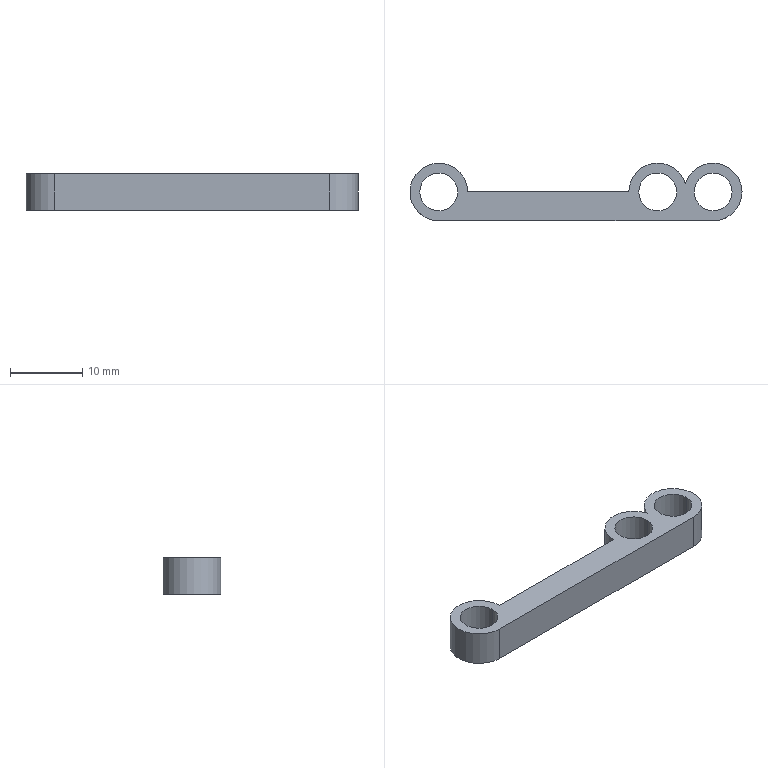Part | SolidWorks | features ICE 13, RevCut 2, Attribute 1, Extrusion 1 | 1 solid | 14 faces | box 46 x 8 x 5 mm | volume 936.72 mm3 | cylinder 10 | plane 4 | commonest cylinder face diameters 5.25 x6 8 x4
STEP:
#1=CARTESIAN_POINT('',(2.051,-2.5,0.));
#2=VERTEX_POINT('',#1);
#3=CARTESIAN_POINT('',(7.301,-2.5,0.));
#4=VERTEX_POINT('',#3);
#5=CARTESIAN_POINT('',(4.676,-2.5,0.));
#6=DIRECTION('',(0.,0.,1.));
#7=DIRECTION('',(1.,0.,0.));
#8=AXIS2_PLACEMENT_3D('',#5,#6,#7);
#9=CIRCLE('',#8,2.625);
#10=EDGE_CURVE('',#2,#4,#9,.T.);
#11=ORIENTED_EDGE('',*,*,#10,.F.);
#12=CARTESIAN_POINT('',(2.051,-2.5,5.));
#13=VERTEX_POINT('',#12);
#14=CARTESIAN_POINT('',(2.051,-2.5,-5.));
#15=DIRECTION('',(0.,0.,1.));
#16=VECTOR('',#15,1000.);
#17=LINE('',#14,#16);
#18=EDGE_CURVE('',#2,#13,#17,.T.);
#19=ORIENTED_EDGE('',*,*,#18,.T.);
#20=CARTESIAN_POINT('',(7.301,-2.5,5.));
#21=VERTEX_POINT('',#20);
#22=CARTESIAN_POINT('',(4.676,-2.5,5.));
#23=DIRECTION('',(0.,0.,1.));
#24=DIRECTION('',(1.,0.,0.));
#25=AXIS2_PLACEMENT_3D('',#22,#23,#24);
#26=CIRCLE('',#25,2.625);
#27=EDGE_CURVE('',#13,#21,#26,.T.);
#28=ORIENTED_EDGE('',*,*,#27,.T.);
#29=CARTESIAN_POINT('',(7.301,-2.5,-5.));
#30=DIRECTION('',(0.,0.,1.));
#31=VECTOR('',#30,1000.);
#32=LINE('',#29,#31);
#33=EDGE_CURVE('',#4,#21,#32,.T.);
#34=ORIENTED_EDGE('',*,*,#33,.F.);
#35=EDGE_LOOP('',(#11,#19,#28,#34));
#36=FACE_OUTER_BOUND('',#35,.T.);
#37=CARTESIAN_POINT('',(4.676,-2.5,-5.));
#38=DIRECTION('',(0.,0.,1.));
#39=DIRECTION('',(1.,0.,0.));
#40=AXIS2_PLACEMENT_3D('',#37,#38,#39);
#41=CYLINDRICAL_SURFACE('',#40,2.625);
#42=ADVANCED_FACE('',(#36),#41,.F.);
#43=CARTESIAN_POINT('',(32.375,-2.5,5.));
#44=VERTEX_POINT('',#43);
#45=CARTESIAN_POINT('',(37.625,-2.5,5.));
#46=VERTEX_POINT('',#45);
#47=CARTESIAN_POINT('',(35.,-2.5,5.));
#48=DIRECTION('',(0.,0.,1.));
#49=DIRECTION('',(1.,0.,0.));
#50=AXIS2_PLACEMENT_3D('',#47,#48,#49);
#51=CIRCLE('',#50,2.625);
#52=EDGE_CURVE('',#44,#46,#51,.T.);
#53=ORIENTED_EDGE('',*,*,#52,.T.);
#54=CARTESIAN_POINT('',(37.625,-2.5,0.));
#55=VERTEX_POINT('',#54);
#56=CARTESIAN_POINT('',(37.625,-2.5,14.));
#57=DIRECTION('',(0.,0.,-1.));
#58=VECTOR('',#57,1000.);
#59=LINE('',#56,#58);
#60=EDGE_CURVE('',#46,#55,#59,.T.);
#61=ORIENTED_EDGE('',*,*,#60,.T.);
#62=CARTESIAN_POINT('',(32.375,-2.5,0.));
#63=VERTEX_POINT('',#62);
#64=CARTESIAN_POINT('',(35.,-2.5,0.));
#65=DIRECTION('',(0.,0.,-1.));
#66=DIRECTION('',(-1.,0.,0.));
#67=AXIS2_PLACEMENT_3D('',#64,#65,#66);
#68=CIRCLE('',#67,2.625);
#69=EDGE_CURVE('',#55,#63,#68,.T.);
#70=ORIENTED_EDGE('',*,*,#69,.T.);
#71=CARTESIAN_POINT('',(32.375,-2.5,14.));
#72=DIRECTION('',(0.,0.,-1.));
#73=VECTOR('',#72,1000.);
#74=LINE('',#71,#73);
#75=EDGE_CURVE('',#44,#63,#74,.T.);
#76=ORIENTED_EDGE('',*,*,#75,.F.);
#77=EDGE_LOOP('',(#53,#61,#70,#76));
#78=FACE_OUTER_BOUND('',#77,.T.);
#79=CARTESIAN_POINT('',(35.,-2.5,14.));
#80=DIRECTION('',(0.,0.,-1.));
#81=DIRECTION('',(-1.,0.,0.));
#82=AXIS2_PLACEMENT_3D('',#79,#80,#81);
#83=CYLINDRICAL_SURFACE('',#82,2.625);
#84=ADVANCED_FACE('',(#78),#83,.F.);
#85=CARTESIAN_POINT('',(40.051,-2.5,0.));
#86=VERTEX_POINT('',#85);
#87=CARTESIAN_POINT('',(45.301,-2.5,0.));
#88=VERTEX_POINT('',#87);
#89=CARTESIAN_POINT('',(42.676,-2.5,0.));
#90=DIRECTION('',(0.,0.,1.));
#91=DIRECTION('',(1.,0.,0.));
#92=AXIS2_PLACEMENT_3D('',#89,#90,#91);
#93=CIRCLE('',#92,2.625);
#94=EDGE_CURVE('',#86,#88,#93,.T.);
#95=ORIENTED_EDGE('',*,*,#94,.F.);
#96=CARTESIAN_POINT('',(40.051,-2.5,5.));
#97=VERTEX_POINT('',#96);
#98=CARTESIAN_POINT('',(40.051,-2.5,-2.));
#99=DIRECTION('',(0.,0.,1.));
#100=VECTOR('',#99,1000.);
#101=LINE('',#98,#100);
#102=EDGE_CURVE('',#86,#97,#101,.T.);
#103=ORIENTED_EDGE('',*,*,#102,.T.);
#104=CARTESIAN_POINT('',(45.301,-2.5,5.));
#105=VERTEX_POINT('',#104);
#106=CARTESIAN_POINT('',(42.676,-2.5,5.));
#107=DIRECTION('',(0.,0.,1.));
#108=DIRECTION('',(1.,0.,0.));
#109=AXIS2_PLACEMENT_3D('',#106,#107,#108);
#110=CIRCLE('',#109,2.625);
#111=EDGE_CURVE('',#97,#105,#110,.T.);
#112=ORIENTED_EDGE('',*,*,#111,.T.);
#113=CARTESIAN_POINT('',(45.301,-2.5,-2.));
#114=DIRECTION('',(0.,0.,1.));
#115=VECTOR('',#114,1000.);
#116=LINE('',#113,#115);
#117=EDGE_CURVE('',#88,#105,#116,.T.);
#118=ORIENTED_EDGE('',*,*,#117,.F.);
#119=EDGE_LOOP('',(#95,#103,#112,#118));
#120=FACE_OUTER_BOUND('',#119,.T.);
#121=CARTESIAN_POINT('',(42.676,-2.5,-2.));
#122=DIRECTION('',(0.,0.,1.));
#123=DIRECTION('',(1.,0.,0.));
#124=AXIS2_PLACEMENT_3D('',#121,#122,#123);
#125=CYLINDRICAL_SURFACE('',#124,2.625);
#126=ADVANCED_FACE('',(#120),#125,.F.);
#127=CARTESIAN_POINT('',(42.676,-6.5,0.));
#128=VERTEX_POINT('',#127);
#129=CARTESIAN_POINT('',(46.676,-2.5,0.));
#130=VERTEX_POINT('',#129);
#131=CARTESIAN_POINT('',(42.676,-2.5,0.));
#132=DIRECTION('',(0.,0.,1.));
#133=DIRECTION('',(1.,0.,0.));
#134=AXIS2_PLACEMENT_3D('',#131,#132,#133);
#135=CIRCLE('',#134,4.);
#136=EDGE_CURVE('',#128,#130,#135,.T.);
#137=ORIENTED_EDGE('',*,*,#136,.T.);
#138=CARTESIAN_POINT('',(46.676,-2.5,5.));
#139=VERTEX_POINT('',#138);
#140=CARTESIAN_POINT('',(46.676,-2.5,0.));
#141=DIRECTION('',(0.,0.,1.));
#142=VECTOR('',#141,1000.);
#143=LINE('',#140,#142);
#144=EDGE_CURVE('',#130,#139,#143,.T.);
#145=ORIENTED_EDGE('',*,*,#144,.T.);
#146=CARTESIAN_POINT('',(42.676,-6.5,5.));
#147=VERTEX_POINT('',#146);
#148=CARTESIAN_POINT('',(42.676,-2.5,5.));
#149=DIRECTION('',(0.,0.,1.));
#150=DIRECTION('',(1.,0.,0.));
#151=AXIS2_PLACEMENT_3D('',#148,#149,#150);
#152=CIRCLE('',#151,4.);
#153=EDGE_CURVE('',#147,#139,#152,.T.);
#154=ORIENTED_EDGE('',*,*,#153,.F.);
#155=CARTESIAN_POINT('',(42.676,-6.5,0.));
#156=DIRECTION('',(0.,0.,1.));
#157=VECTOR('',#156,1000.);
#158=LINE('',#155,#157);
#159=EDGE_CURVE('',#128,#147,#158,.T.);
#160=ORIENTED_EDGE('',*,*,#159,.F.);
#161=EDGE_LOOP('',(#137,#145,#154,#160));
#162=FACE_OUTER_BOUND('',#161,.T.);
#163=CARTESIAN_POINT('',(42.676,-2.5,0.));
#164=DIRECTION('',(0.,0.,1.));
#165=DIRECTION('',(1.,0.,0.));
#166=AXIS2_PLACEMENT_3D('',#163,#164,#165);
#167=CYLINDRICAL_SURFACE('',#166,4.);
#168=ADVANCED_FACE('',(#162),#167,.T.);
#169=ORIENTED_EDGE('',*,*,#144,.F.);
#170=CARTESIAN_POINT('',(38.838,-1.373,0.));
#171=VERTEX_POINT('',#170);
#172=CARTESIAN_POINT('',(42.676,-2.5,0.));
#173=DIRECTION('',(0.,0.,1.));
#174=DIRECTION('',(1.,0.,0.));
#175=AXIS2_PLACEMENT_3D('',#172,#173,#174);
#176=CIRCLE('',#175,4.);
#177=EDGE_CURVE('',#130,#171,#176,.T.);
#178=ORIENTED_EDGE('',*,*,#177,.T.);
#179=CARTESIAN_POINT('',(38.838,-1.373,5.));
#180=VERTEX_POINT('',#179);
#181=CARTESIAN_POINT('',(38.838,-1.373,0.));
#182=DIRECTION('',(0.,0.,1.));
#183=VECTOR('',#182,1000.);
#184=LINE('',#181,#183);
#185=EDGE_CURVE('',#171,#180,#184,.T.);
#186=ORIENTED_EDGE('',*,*,#185,.T.);
#187=CARTESIAN_POINT('',(42.676,-2.5,5.));
#188=DIRECTION('',(0.,0.,1.));
#189=DIRECTION('',(1.,0.,0.));
#190=AXIS2_PLACEMENT_3D('',#187,#188,#189);
#191=CIRCLE('',#190,4.);
#192=EDGE_CURVE('',#139,#180,#191,.T.);
#193=ORIENTED_EDGE('',*,*,#192,.F.);
#194=EDGE_LOOP('',(#169,#178,#186,#193));
#195=FACE_OUTER_BOUND('',#194,.T.);
#196=CARTESIAN_POINT('',(42.676,-2.5,0.));
#197=DIRECTION('',(0.,0.,1.));
#198=DIRECTION('',(1.,0.,0.));
#199=AXIS2_PLACEMENT_3D('',#196,#197,#198);
#200=CYLINDRICAL_SURFACE('',#199,4.);
#201=ADVANCED_FACE('',(#195),#200,.T.);
#202=CARTESIAN_POINT('',(8.676,-2.5,5.));
#203=VERTEX_POINT('',#202);
#204=CARTESIAN_POINT('',(4.676,-6.5,5.));
#205=VERTEX_POINT('',#204);
#206=CARTESIAN_POINT('',(4.676,-2.5,5.));
#207=DIRECTION('',(0.,0.,1.));
#208=DIRECTION('',(1.,0.,0.));
#209=AXIS2_PLACEMENT_3D('',#206,#207,#208);
#210=CIRCLE('',#209,4.);
#211=EDGE_CURVE('',#203,#205,#210,.T.);
#212=ORIENTED_EDGE('',*,*,#211,.T.);
#213=CARTESIAN_POINT('',(35.,-6.5,5.));
#214=DIRECTION('',(1.,0.,0.));
#215=VECTOR('',#214,1000.);
#216=LINE('',#213,#215);
#217=EDGE_CURVE('',#205,#147,#216,.T.);
#218=ORIENTED_EDGE('',*,*,#217,.T.);
#219=ORIENTED_EDGE('',*,*,#153,.T.);
#220=ORIENTED_EDGE('',*,*,#192,.T.);
#221=CARTESIAN_POINT('',(31.,-2.5,5.));
#222=VERTEX_POINT('',#221);
#223=CARTESIAN_POINT('',(35.,-2.5,5.));
#224=DIRECTION('',(0.,0.,-1.));
#225=DIRECTION('',(-1.,0.,0.));
#226=AXIS2_PLACEMENT_3D('',#223,#224,#225);
#227=CIRCLE('',#226,4.);
#228=EDGE_CURVE('',#222,#180,#227,.T.);
#229=ORIENTED_EDGE('',*,*,#228,.F.);
#230=CARTESIAN_POINT('',(0.,-2.5,5.));
#231=DIRECTION('',(1.,0.,0.));
#232=VECTOR('',#231,1000.);
#233=LINE('',#230,#232);
#234=EDGE_CURVE('',#203,#222,#233,.T.);
#235=ORIENTED_EDGE('',*,*,#234,.F.);
#236=EDGE_LOOP('',(#212,#218,#219,#220,#229,#235));
#237=FACE_OUTER_BOUND('',#236,.T.);
#238=CARTESIAN_POINT('',(4.676,-2.5,5.));
#239=DIRECTION('',(0.,0.,1.));
#240=DIRECTION('',(1.,0.,0.));
#241=AXIS2_PLACEMENT_3D('',#238,#239,#240);
#242=CIRCLE('',#241,2.625);
#243=EDGE_CURVE('',#21,#13,#242,.T.);
#244=ORIENTED_EDGE('',*,*,#243,.F.);
#245=ORIENTED_EDGE('',*,*,#27,.F.);
#246=EDGE_LOOP('',(#244,#245));
#247=FACE_BOUND('',#246,.T.);
#248=ORIENTED_EDGE('',*,*,#52,.F.);
#249=CARTESIAN_POINT('',(35.,-2.5,5.));
#250=DIRECTION('',(0.,0.,1.));
#251=DIRECTION('',(1.,0.,0.));
#252=AXIS2_PLACEMENT_3D('',#249,#250,#251);
#253=CIRCLE('',#252,2.625);
#254=EDGE_CURVE('',#46,#44,#253,.T.);
#255=ORIENTED_EDGE('',*,*,#254,.F.);
#256=EDGE_LOOP('',(#248,#255));
#257=FACE_BOUND('',#256,.T.);
#258=CARTESIAN_POINT('',(42.676,-2.5,5.));
#259=DIRECTION('',(0.,0.,1.));
#260=DIRECTION('',(1.,0.,0.));
#261=AXIS2_PLACEMENT_3D('',#258,#259,#260);
#262=CIRCLE('',#261,2.625);
#263=EDGE_CURVE('',#105,#97,#262,.T.);
#264=ORIENTED_EDGE('',*,*,#263,.F.);
#265=ORIENTED_EDGE('',*,*,#111,.F.);
#266=EDGE_LOOP('',(#264,#265));
#267=FACE_BOUND('',#266,.T.);
#268=CARTESIAN_POINT('',(44.,-1.,5.));
#269=DIRECTION('',(0.,0.,1.));
#270=DIRECTION('',(1.,0.,0.));
#271=AXIS2_PLACEMENT_3D('',#268,#269,#270);
#272=PLANE('',#271);
#273=ADVANCED_FACE('',(#237,#247,#257,#267),#272,.T.);
#274=CARTESIAN_POINT('',(4.676,-6.5,0.));
#275=VERTEX_POINT('',#274);
#276=CARTESIAN_POINT('',(4.676,-6.5,0.));
#277=DIRECTION('',(1.,0.,0.));
#278=VECTOR('',#277,1000.);
#279=LINE('',#276,#278);
#280=EDGE_CURVE('',#275,#128,#279,.T.);
#281=ORIENTED_EDGE('',*,*,#280,.F.);
#282=CARTESIAN_POINT('',(8.676,-2.5,0.));
#283=VERTEX_POINT('',#282);
#284=CARTESIAN_POINT('',(4.676,-2.5,0.));
#285=DIRECTION('',(0.,0.,1.));
#286=DIRECTION('',(1.,0.,0.));
#287=AXIS2_PLACEMENT_3D('',#284,#285,#286);
#288=CIRCLE('',#287,4.);
#289=EDGE_CURVE('',#283,#275,#288,.T.);
#290=ORIENTED_EDGE('',*,*,#289,.F.);
#291=CARTESIAN_POINT('',(31.,-2.5,0.));
#292=VERTEX_POINT('',#291);
#293=CARTESIAN_POINT('',(0.,-2.5,0.));
#294=DIRECTION('',(1.,0.,0.));
#295=VECTOR('',#294,1000.);
#296=LINE('',#293,#295);
#297=EDGE_CURVE('',#283,#292,#296,.T.);
#298=ORIENTED_EDGE('',*,*,#297,.T.);
#299=CARTESIAN_POINT('',(35.,-2.5,0.));
#300=DIRECTION('',(0.,0.,-1.));
#301=DIRECTION('',(-1.,0.,0.));
#302=AXIS2_PLACEMENT_3D('',#299,#300,#301);
#303=CIRCLE('',#302,4.);
#304=EDGE_CURVE('',#292,#171,#303,.T.);
#305=ORIENTED_EDGE('',*,*,#304,.T.);
#306=ORIENTED_EDGE('',*,*,#177,.F.);
#307=ORIENTED_EDGE('',*,*,#136,.F.);
#308=EDGE_LOOP('',(#281,#290,#298,#305,#306,#307));
#309=FACE_OUTER_BOUND('',#308,.T.);
#310=CARTESIAN_POINT('',(4.676,-2.5,0.));
#311=DIRECTION('',(0.,0.,1.));
#312=DIRECTION('',(1.,0.,0.));
#313=AXIS2_PLACEMENT_3D('',#310,#311,#312);
#314=CIRCLE('',#313,2.625);
#315=EDGE_CURVE('',#4,#2,#314,.T.);
#316=ORIENTED_EDGE('',*,*,#315,.T.);
#317=ORIENTED_EDGE('',*,*,#10,.T.);
#318=EDGE_LOOP('',(#316,#317));
#319=FACE_BOUND('',#318,.T.);
#320=CARTESIAN_POINT('',(35.,-2.5,0.));
#321=DIRECTION('',(0.,0.,-1.));
#322=DIRECTION('',(-1.,0.,0.));
#323=AXIS2_PLACEMENT_3D('',#320,#321,#322);
#324=CIRCLE('',#323,2.625);
#325=EDGE_CURVE('',#63,#55,#324,.T.);
#326=ORIENTED_EDGE('',*,*,#325,.F.);
#327=ORIENTED_EDGE('',*,*,#69,.F.);
#328=EDGE_LOOP('',(#326,#327));
#329=FACE_BOUND('',#328,.T.);
#330=CARTESIAN_POINT('',(42.676,-2.5,0.));
#331=DIRECTION('',(0.,0.,1.));
#332=DIRECTION('',(1.,0.,0.));
#333=AXIS2_PLACEMENT_3D('',#330,#331,#332);
#334=CIRCLE('',#333,2.625);
#335=EDGE_CURVE('',#88,#86,#334,.T.);
#336=ORIENTED_EDGE('',*,*,#335,.T.);
#337=ORIENTED_EDGE('',*,*,#94,.T.);
#338=EDGE_LOOP('',(#336,#337));
#339=FACE_BOUND('',#338,.T.);
#340=CARTESIAN_POINT('',(44.,-1.,0.));
#341=DIRECTION('',(0.,0.,1.));
#342=DIRECTION('',(1.,0.,0.));
#343=AXIS2_PLACEMENT_3D('',#340,#341,#342);
#344=PLANE('',#343);
#345=ADVANCED_FACE('',(#309,#319,#329,#339),#344,.F.);
#346=ORIENTED_EDGE('',*,*,#102,.F.);
#347=ORIENTED_EDGE('',*,*,#335,.F.);
#348=ORIENTED_EDGE('',*,*,#117,.T.);
#349=ORIENTED_EDGE('',*,*,#263,.T.);
#350=EDGE_LOOP('',(#346,#347,#348,#349));
#351=FACE_OUTER_BOUND('',#350,.T.);
#352=CARTESIAN_POINT('',(42.676,-2.5,-2.));
#353=DIRECTION('',(0.,0.,1.));
#354=DIRECTION('',(1.,0.,0.));
#355=AXIS2_PLACEMENT_3D('',#352,#353,#354);
#356=CYLINDRICAL_SURFACE('',#355,2.625);
#357=ADVANCED_FACE('',(#351),#356,.F.);
#358=ORIENTED_EDGE('',*,*,#304,.F.);
#359=CARTESIAN_POINT('',(31.,-2.5,0.));
#360=DIRECTION('',(0.,0.,1.));
#361=VECTOR('',#360,1000.);
#362=LINE('',#359,#361);
#363=EDGE_CURVE('',#292,#222,#362,.T.);
#364=ORIENTED_EDGE('',*,*,#363,.T.);
#365=ORIENTED_EDGE('',*,*,#228,.T.);
#366=ORIENTED_EDGE('',*,*,#185,.F.);
#367=EDGE_LOOP('',(#358,#364,#365,#366));
#368=FACE_OUTER_BOUND('',#367,.T.);
#369=CARTESIAN_POINT('',(35.,-2.5,5.));
#370=DIRECTION('',(0.,0.,-1.));
#371=DIRECTION('',(-1.,0.,0.));
#372=AXIS2_PLACEMENT_3D('',#369,#370,#371);
#373=CYLINDRICAL_SURFACE('',#372,4.);
#374=ADVANCED_FACE('',(#368),#373,.T.);
#375=ORIENTED_EDGE('',*,*,#60,.F.);
#376=ORIENTED_EDGE('',*,*,#254,.T.);
#377=ORIENTED_EDGE('',*,*,#75,.T.);
#378=ORIENTED_EDGE('',*,*,#325,.T.);
#379=EDGE_LOOP('',(#375,#376,#377,#378));
#380=FACE_OUTER_BOUND('',#379,.T.);
#381=CARTESIAN_POINT('',(35.,-2.5,14.));
#382=DIRECTION('',(0.,0.,-1.));
#383=DIRECTION('',(-1.,0.,0.));
#384=AXIS2_PLACEMENT_3D('',#381,#382,#383);
#385=CYLINDRICAL_SURFACE('',#384,2.625);
#386=ADVANCED_FACE('',(#380),#385,.F.);
#387=CARTESIAN_POINT('',(4.676,-6.5,0.));
#388=DIRECTION('',(0.,0.,1.));
#389=VECTOR('',#388,1000.);
#390=LINE('',#387,#389);
#391=EDGE_CURVE('',#275,#205,#390,.T.);
#392=ORIENTED_EDGE('',*,*,#391,.T.);
#393=ORIENTED_EDGE('',*,*,#211,.F.);
#394=CARTESIAN_POINT('',(8.676,-2.5,0.));
#395=DIRECTION('',(0.,0.,1.));
#396=VECTOR('',#395,1000.);
#397=LINE('',#394,#396);
#398=EDGE_CURVE('',#283,#203,#397,.T.);
#399=ORIENTED_EDGE('',*,*,#398,.F.);
#400=ORIENTED_EDGE('',*,*,#289,.T.);
#401=EDGE_LOOP('',(#392,#393,#399,#400));
#402=FACE_OUTER_BOUND('',#401,.T.);
#403=CARTESIAN_POINT('',(4.676,-2.5,0.));
#404=DIRECTION('',(0.,0.,1.));
#405=DIRECTION('',(1.,0.,0.));
#406=AXIS2_PLACEMENT_3D('',#403,#404,#405);
#407=CYLINDRICAL_SURFACE('',#406,4.);
#408=ADVANCED_FACE('',(#402),#407,.T.);
#409=ORIENTED_EDGE('',*,*,#18,.F.);
#410=ORIENTED_EDGE('',*,*,#315,.F.);
#411=ORIENTED_EDGE('',*,*,#33,.T.);
#412=ORIENTED_EDGE('',*,*,#243,.T.);
#413=EDGE_LOOP('',(#409,#410,#411,#412));
#414=FACE_OUTER_BOUND('',#413,.T.);
#415=CARTESIAN_POINT('',(4.676,-2.5,-5.));
#416=DIRECTION('',(0.,0.,1.));
#417=DIRECTION('',(1.,0.,0.));
#418=AXIS2_PLACEMENT_3D('',#415,#416,#417);
#419=CYLINDRICAL_SURFACE('',#418,2.625);
#420=ADVANCED_FACE('',(#414),#419,.F.);
#421=ORIENTED_EDGE('',*,*,#234,.T.);
#422=ORIENTED_EDGE('',*,*,#363,.F.);
#423=ORIENTED_EDGE('',*,*,#297,.F.);
#424=ORIENTED_EDGE('',*,*,#398,.T.);
#425=EDGE_LOOP('',(#421,#422,#423,#424));
#426=FACE_OUTER_BOUND('',#425,.T.);
#427=CARTESIAN_POINT('',(0.,-2.5,0.));
#428=DIRECTION('',(0.,-1.,0.));
#429=DIRECTION('',(1.,0.,0.));
#430=AXIS2_PLACEMENT_3D('',#427,#428,#429);
#431=PLANE('',#430);
#432=ADVANCED_FACE('',(#426),#431,.F.);
#433=ORIENTED_EDGE('',*,*,#217,.F.);
#434=ORIENTED_EDGE('',*,*,#391,.F.);
#435=ORIENTED_EDGE('',*,*,#280,.T.);
#436=ORIENTED_EDGE('',*,*,#159,.T.);
#437=EDGE_LOOP('',(#433,#434,#435,#436));
#438=FACE_OUTER_BOUND('',#437,.T.);
#439=CARTESIAN_POINT('',(35.,-6.5,0.));
#440=DIRECTION('',(0.,-1.,0.));
#441=DIRECTION('',(0.,0.,-1.));
#442=AXIS2_PLACEMENT_3D('',#439,#440,#441);
#443=PLANE('',#442);
#444=ADVANCED_FACE('',(#438),#443,.T.);
#445=CLOSED_SHELL('',(#42,#84,#126,#168,#201,#273,#345,#357,#374,#386,#408,#420,#432,#444));
#446=MANIFOLD_SOLID_BREP('',#445);
#447=CARTESIAN_POINT('',(0.,0.,0.));
#448=DIRECTION('',(0.,0.,1.));
#449=DIRECTION('',(1.,0.,0.));
#450=AXIS2_PLACEMENT_3D('',#447,#448,#449);
#451=(LENGTH_UNIT()NAMED_UNIT(*)SI_UNIT(.MILLI.,.METRE.));
#452=UNCERTAINTY_MEASURE_WITH_UNIT(LENGTH_MEASURE(0.00001),#451,'','');
#453=(NAMED_UNIT(*)PLANE_ANGLE_UNIT()SI_UNIT($,.RADIAN.));
#454=(NAMED_UNIT(*)SI_UNIT($,.STERADIAN.)SOLID_ANGLE_UNIT());
#455=(GEOMETRIC_REPRESENTATION_CONTEXT(3)GLOBAL_UNCERTAINTY_ASSIGNED_CONTEXT((#452))GLOBAL_UNIT_ASSIGNED_CONTEXT((#451,#453,#454))REPRESENTATION_CONTEXT('',''));
#456=ADVANCED_BREP_SHAPE_REPRESENTATION('',(#446,#450),#455);